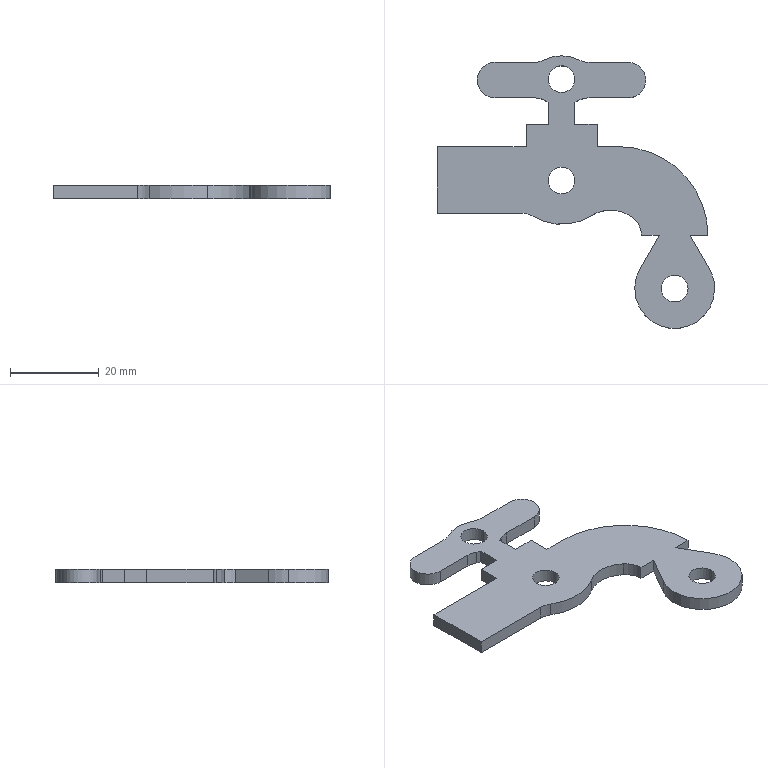Part | SolidWorks | features FlatPattern 1, ICE 1, SMBaseFlange 1, SheetMetal 1 | 1 solid | 44 faces | box 62.5 x 61.5 x 3 mm | volume 4665 mm3 | cylinder 24 | plane 20 | commonest cylinder face diameters 6 x6 10 x6 8 x3 17 x3 18 x3 16.181 x1
STEP:
#1=CARTESIAN_POINT('',(25.,30.211,-3.));
#2=VERTEX_POINT('',#1);
#3=CARTESIAN_POINT('',(31.,30.211,-3.));
#4=VERTEX_POINT('',#3);
#5=CARTESIAN_POINT('',(28.,30.211,-3.));
#6=DIRECTION('',(0.,0.,1.));
#7=DIRECTION('',(1.,0.,0.));
#8=AXIS2_PLACEMENT_3D('',#5,#6,#7);
#9=CIRCLE('',#8,3.);
#10=EDGE_CURVE('',#2,#4,#9,.T.);
#11=ORIENTED_EDGE('',*,*,#10,.F.);
#12=CARTESIAN_POINT('',(25.,30.211,0.));
#13=VERTEX_POINT('',#12);
#14=CARTESIAN_POINT('',(25.,30.211,-10.));
#15=DIRECTION('',(0.,0.,1.));
#16=VECTOR('',#15,1000.);
#17=LINE('',#14,#16);
#18=EDGE_CURVE('',#2,#13,#17,.T.);
#19=ORIENTED_EDGE('',*,*,#18,.T.);
#20=CARTESIAN_POINT('',(31.,30.211,0.));
#21=VERTEX_POINT('',#20);
#22=CARTESIAN_POINT('',(28.,30.211,0.));
#23=DIRECTION('',(0.,0.,1.));
#24=DIRECTION('',(1.,0.,0.));
#25=AXIS2_PLACEMENT_3D('',#22,#23,#24);
#26=CIRCLE('',#25,3.);
#27=EDGE_CURVE('',#13,#21,#26,.T.);
#28=ORIENTED_EDGE('',*,*,#27,.T.);
#29=CARTESIAN_POINT('',(31.,30.211,-10.));
#30=DIRECTION('',(0.,0.,1.));
#31=VECTOR('',#30,1000.);
#32=LINE('',#29,#31);
#33=EDGE_CURVE('',#4,#21,#32,.T.);
#34=ORIENTED_EDGE('',*,*,#33,.F.);
#35=EDGE_LOOP('',(#11,#19,#28,#34));
#36=FACE_OUTER_BOUND('',#35,.T.);
#37=CARTESIAN_POINT('',(28.,30.211,-10.));
#38=DIRECTION('',(0.,0.,1.));
#39=DIRECTION('',(1.,0.,0.));
#40=AXIS2_PLACEMENT_3D('',#37,#38,#39);
#41=CYLINDRICAL_SURFACE('',#40,3.);
#42=ADVANCED_FACE('',(#36),#41,.F.);
#43=CARTESIAN_POINT('',(25.,7.369,-3.));
#44=VERTEX_POINT('',#43);
#45=CARTESIAN_POINT('',(31.,7.369,-3.));
#46=VERTEX_POINT('',#45);
#47=CARTESIAN_POINT('',(28.,7.369,-3.));
#48=DIRECTION('',(0.,0.,1.));
#49=DIRECTION('',(1.,0.,0.));
#50=AXIS2_PLACEMENT_3D('',#47,#48,#49);
#51=CIRCLE('',#50,3.);
#52=EDGE_CURVE('',#44,#46,#51,.T.);
#53=ORIENTED_EDGE('',*,*,#52,.F.);
#54=CARTESIAN_POINT('',(25.,7.369,0.));
#55=VERTEX_POINT('',#54);
#56=CARTESIAN_POINT('',(25.,7.369,-10.));
#57=DIRECTION('',(0.,0.,1.));
#58=VECTOR('',#57,1000.);
#59=LINE('',#56,#58);
#60=EDGE_CURVE('',#44,#55,#59,.T.);
#61=ORIENTED_EDGE('',*,*,#60,.T.);
#62=CARTESIAN_POINT('',(31.,7.369,0.));
#63=VERTEX_POINT('',#62);
#64=CARTESIAN_POINT('',(28.,7.369,0.));
#65=DIRECTION('',(0.,0.,1.));
#66=DIRECTION('',(1.,0.,0.));
#67=AXIS2_PLACEMENT_3D('',#64,#65,#66);
#68=CIRCLE('',#67,3.);
#69=EDGE_CURVE('',#55,#63,#68,.T.);
#70=ORIENTED_EDGE('',*,*,#69,.T.);
#71=CARTESIAN_POINT('',(31.,7.369,-10.));
#72=DIRECTION('',(0.,0.,1.));
#73=VECTOR('',#72,1000.);
#74=LINE('',#71,#73);
#75=EDGE_CURVE('',#46,#63,#74,.T.);
#76=ORIENTED_EDGE('',*,*,#75,.F.);
#77=EDGE_LOOP('',(#53,#61,#70,#76));
#78=FACE_OUTER_BOUND('',#77,.T.);
#79=CARTESIAN_POINT('',(28.,7.369,-10.));
#80=DIRECTION('',(0.,0.,1.));
#81=DIRECTION('',(1.,0.,0.));
#82=AXIS2_PLACEMENT_3D('',#79,#80,#81);
#83=CYLINDRICAL_SURFACE('',#82,3.);
#84=ADVANCED_FACE('',(#78),#83,.F.);
#85=CARTESIAN_POINT('',(50.5,-17.,-3.));
#86=VERTEX_POINT('',#85);
#87=CARTESIAN_POINT('',(56.5,-17.,-3.));
#88=VERTEX_POINT('',#87);
#89=CARTESIAN_POINT('',(53.5,-17.,-3.));
#90=DIRECTION('',(0.,0.,1.));
#91=DIRECTION('',(1.,0.,0.));
#92=AXIS2_PLACEMENT_3D('',#89,#90,#91);
#93=CIRCLE('',#92,3.);
#94=EDGE_CURVE('',#86,#88,#93,.T.);
#95=ORIENTED_EDGE('',*,*,#94,.F.);
#96=CARTESIAN_POINT('',(50.5,-17.,0.));
#97=VERTEX_POINT('',#96);
#98=CARTESIAN_POINT('',(50.5,-17.,-10.));
#99=DIRECTION('',(0.,0.,1.));
#100=VECTOR('',#99,1000.);
#101=LINE('',#98,#100);
#102=EDGE_CURVE('',#86,#97,#101,.T.);
#103=ORIENTED_EDGE('',*,*,#102,.T.);
#104=CARTESIAN_POINT('',(56.5,-17.,0.));
#105=VERTEX_POINT('',#104);
#106=CARTESIAN_POINT('',(53.5,-17.,0.));
#107=DIRECTION('',(0.,0.,1.));
#108=DIRECTION('',(1.,0.,0.));
#109=AXIS2_PLACEMENT_3D('',#106,#107,#108);
#110=CIRCLE('',#109,3.);
#111=EDGE_CURVE('',#97,#105,#110,.T.);
#112=ORIENTED_EDGE('',*,*,#111,.T.);
#113=CARTESIAN_POINT('',(56.5,-17.,-10.));
#114=DIRECTION('',(0.,0.,1.));
#115=VECTOR('',#114,1000.);
#116=LINE('',#113,#115);
#117=EDGE_CURVE('',#88,#105,#116,.T.);
#118=ORIENTED_EDGE('',*,*,#117,.F.);
#119=EDGE_LOOP('',(#95,#103,#112,#118));
#120=FACE_OUTER_BOUND('',#119,.T.);
#121=CARTESIAN_POINT('',(53.5,-17.,-10.));
#122=DIRECTION('',(0.,0.,1.));
#123=DIRECTION('',(1.,0.,0.));
#124=AXIS2_PLACEMENT_3D('',#121,#122,#123);
#125=CYLINDRICAL_SURFACE('',#124,3.);
#126=ADVANCED_FACE('',(#120),#125,.F.);
#127=CARTESIAN_POINT('',(45.706,-12.5,-3.));
#128=VERTEX_POINT('',#127);
#129=CARTESIAN_POINT('',(44.5,-17.,-3.));
#130=VERTEX_POINT('',#129);
#131=CARTESIAN_POINT('',(53.5,-17.,-3.));
#132=DIRECTION('',(0.,0.,1.));
#133=DIRECTION('',(1.,0.,0.));
#134=AXIS2_PLACEMENT_3D('',#131,#132,#133);
#135=CIRCLE('',#134,9.);
#136=EDGE_CURVE('',#128,#130,#135,.T.);
#137=ORIENTED_EDGE('',*,*,#136,.T.);
#138=CARTESIAN_POINT('',(44.5,-17.,0.));
#139=VERTEX_POINT('',#138);
#140=CARTESIAN_POINT('',(44.5,-17.,-3.));
#141=DIRECTION('',(0.,0.,1.));
#142=VECTOR('',#141,1000.);
#143=LINE('',#140,#142);
#144=EDGE_CURVE('',#130,#139,#143,.T.);
#145=ORIENTED_EDGE('',*,*,#144,.T.);
#146=CARTESIAN_POINT('',(45.706,-12.5,0.));
#147=VERTEX_POINT('',#146);
#148=CARTESIAN_POINT('',(53.5,-17.,0.));
#149=DIRECTION('',(0.,0.,1.));
#150=DIRECTION('',(1.,0.,0.));
#151=AXIS2_PLACEMENT_3D('',#148,#149,#150);
#152=CIRCLE('',#151,9.);
#153=EDGE_CURVE('',#147,#139,#152,.T.);
#154=ORIENTED_EDGE('',*,*,#153,.F.);
#155=CARTESIAN_POINT('',(45.706,-12.5,-3.));
#156=DIRECTION('',(0.,0.,1.));
#157=VECTOR('',#156,1000.);
#158=LINE('',#155,#157);
#159=EDGE_CURVE('',#128,#147,#158,.T.);
#160=ORIENTED_EDGE('',*,*,#159,.F.);
#161=EDGE_LOOP('',(#137,#145,#154,#160));
#162=FACE_OUTER_BOUND('',#161,.T.);
#163=CARTESIAN_POINT('',(53.5,-17.,-3.));
#164=DIRECTION('',(0.,0.,1.));
#165=DIRECTION('',(1.,0.,0.));
#166=AXIS2_PLACEMENT_3D('',#163,#164,#165);
#167=CYLINDRICAL_SURFACE('',#166,9.);
#168=ADVANCED_FACE('',(#162),#167,.T.);
#169=ORIENTED_EDGE('',*,*,#144,.F.);
#170=CARTESIAN_POINT('',(62.5,-17.,-3.));
#171=VERTEX_POINT('',#170);
#172=CARTESIAN_POINT('',(53.5,-17.,-3.));
#173=DIRECTION('',(0.,0.,1.));
#174=DIRECTION('',(1.,0.,0.));
#175=AXIS2_PLACEMENT_3D('',#172,#173,#174);
#176=CIRCLE('',#175,9.);
#177=EDGE_CURVE('',#130,#171,#176,.T.);
#178=ORIENTED_EDGE('',*,*,#177,.T.);
#179=CARTESIAN_POINT('',(62.5,-17.,0.));
#180=VERTEX_POINT('',#179);
#181=CARTESIAN_POINT('',(62.5,-17.,-3.));
#182=DIRECTION('',(0.,0.,1.));
#183=VECTOR('',#182,1000.);
#184=LINE('',#181,#183);
#185=EDGE_CURVE('',#171,#180,#184,.T.);
#186=ORIENTED_EDGE('',*,*,#185,.T.);
#187=CARTESIAN_POINT('',(53.5,-17.,0.));
#188=DIRECTION('',(0.,0.,1.));
#189=DIRECTION('',(1.,0.,0.));
#190=AXIS2_PLACEMENT_3D('',#187,#188,#189);
#191=CIRCLE('',#190,9.);
#192=EDGE_CURVE('',#139,#180,#191,.T.);
#193=ORIENTED_EDGE('',*,*,#192,.F.);
#194=EDGE_LOOP('',(#169,#178,#186,#193));
#195=FACE_OUTER_BOUND('',#194,.T.);
#196=CARTESIAN_POINT('',(53.5,-17.,-3.));
#197=DIRECTION('',(0.,0.,1.));
#198=DIRECTION('',(1.,0.,0.));
#199=AXIS2_PLACEMENT_3D('',#196,#197,#198);
#200=CYLINDRICAL_SURFACE('',#199,9.);
#201=ADVANCED_FACE('',(#195),#200,.T.);
#202=CARTESIAN_POINT('',(43.,26.,-3.));
#203=VERTEX_POINT('',#202);
#204=CARTESIAN_POINT('',(47.,30.,-3.));
#205=VERTEX_POINT('',#204);
#206=CARTESIAN_POINT('',(43.,30.,-3.));
#207=DIRECTION('',(0.,0.,1.));
#208=DIRECTION('',(1.,0.,0.));
#209=AXIS2_PLACEMENT_3D('',#206,#207,#208);
#210=CIRCLE('',#209,4.);
#211=EDGE_CURVE('',#203,#205,#210,.T.);
#212=ORIENTED_EDGE('',*,*,#211,.T.);
#213=CARTESIAN_POINT('',(47.,30.,0.));
#214=VERTEX_POINT('',#213);
#215=CARTESIAN_POINT('',(47.,30.,-3.));
#216=DIRECTION('',(0.,0.,1.));
#217=VECTOR('',#216,1000.);
#218=LINE('',#215,#217);
#219=EDGE_CURVE('',#205,#214,#218,.T.);
#220=ORIENTED_EDGE('',*,*,#219,.T.);
#221=CARTESIAN_POINT('',(43.,26.,0.));
#222=VERTEX_POINT('',#221);
#223=CARTESIAN_POINT('',(43.,30.,0.));
#224=DIRECTION('',(0.,0.,1.));
#225=DIRECTION('',(1.,0.,0.));
#226=AXIS2_PLACEMENT_3D('',#223,#224,#225);
#227=CIRCLE('',#226,4.);
#228=EDGE_CURVE('',#222,#214,#227,.T.);
#229=ORIENTED_EDGE('',*,*,#228,.F.);
#230=CARTESIAN_POINT('',(43.,26.,-3.));
#231=DIRECTION('',(0.,0.,1.));
#232=VECTOR('',#231,1000.);
#233=LINE('',#230,#232);
#234=EDGE_CURVE('',#203,#222,#233,.T.);
#235=ORIENTED_EDGE('',*,*,#234,.F.);
#236=EDGE_LOOP('',(#212,#220,#229,#235));
#237=FACE_OUTER_BOUND('',#236,.T.);
#238=CARTESIAN_POINT('',(43.,30.,-3.));
#239=DIRECTION('',(0.,0.,1.));
#240=DIRECTION('',(1.,0.,0.));
#241=AXIS2_PLACEMENT_3D('',#238,#239,#240);
#242=CYLINDRICAL_SURFACE('',#241,4.);
#243=ADVANCED_FACE('',(#237),#242,.T.);
#244=CARTESIAN_POINT('',(0.,0.,0.));
#245=VERTEX_POINT('',#244);
#246=CARTESIAN_POINT('',(18.986,0.,0.));
#247=VERTEX_POINT('',#246);
#248=CARTESIAN_POINT('',(0.,0.,0.));
#249=DIRECTION('',(1.,0.,0.));
#250=VECTOR('',#249,1000.);
#251=LINE('',#248,#250);
#252=EDGE_CURVE('',#245,#247,#251,.T.);
#253=ORIENTED_EDGE('',*,*,#252,.F.);
#254=CARTESIAN_POINT('',(0.,0.,-3.));
#255=VERTEX_POINT('',#254);
#256=CARTESIAN_POINT('',(0.,0.,-3.));
#257=DIRECTION('',(0.,0.,1.));
#258=VECTOR('',#257,1000.);
#259=LINE('',#256,#258);
#260=EDGE_CURVE('',#255,#245,#259,.T.);
#261=ORIENTED_EDGE('',*,*,#260,.F.);
#262=CARTESIAN_POINT('',(18.986,0.,-3.));
#263=VERTEX_POINT('',#262);
#264=CARTESIAN_POINT('',(0.,0.,-3.));
#265=DIRECTION('',(1.,0.,0.));
#266=VECTOR('',#265,1000.);
#267=LINE('',#264,#266);
#268=EDGE_CURVE('',#255,#263,#267,.T.);
#269=ORIENTED_EDGE('',*,*,#268,.T.);
#270=CARTESIAN_POINT('',(18.986,0.,-3.));
#271=DIRECTION('',(0.,0.,1.));
#272=VECTOR('',#271,1000.);
#273=LINE('',#270,#272);
#274=EDGE_CURVE('',#263,#247,#273,.T.);
#275=ORIENTED_EDGE('',*,*,#274,.T.);
#276=EDGE_LOOP('',(#253,#261,#269,#275));
#277=FACE_OUTER_BOUND('',#276,.T.);
#278=CARTESIAN_POINT('',(0.,0.,-3.));
#279=DIRECTION('',(0.,-1.,0.));
#280=DIRECTION('',(0.,0.,-1.));
#281=AXIS2_PLACEMENT_3D('',#278,#279,#280);
#282=PLANE('',#281);
#283=ADVANCED_FACE('',(#277),#282,.T.);
#284=CARTESIAN_POINT('',(0.,15.,0.));
#285=VERTEX_POINT('',#284);
#286=CARTESIAN_POINT('',(0.,0.,0.));
#287=DIRECTION('',(0.,-1.,0.));
#288=VECTOR('',#287,1000.);
#289=LINE('',#286,#288);
#290=EDGE_CURVE('',#285,#245,#289,.T.);
#291=ORIENTED_EDGE('',*,*,#290,.F.);
#292=CARTESIAN_POINT('',(0.,15.,-3.));
#293=VERTEX_POINT('',#292);
#294=CARTESIAN_POINT('',(0.,15.,-3.));
#295=DIRECTION('',(0.,0.,1.));
#296=VECTOR('',#295,1000.);
#297=LINE('',#294,#296);
#298=EDGE_CURVE('',#293,#285,#297,.T.);
#299=ORIENTED_EDGE('',*,*,#298,.F.);
#300=CARTESIAN_POINT('',(0.,0.,-3.));
#301=DIRECTION('',(0.,-1.,0.));
#302=VECTOR('',#301,1000.);
#303=LINE('',#300,#302);
#304=EDGE_CURVE('',#293,#255,#303,.T.);
#305=ORIENTED_EDGE('',*,*,#304,.T.);
#306=ORIENTED_EDGE('',*,*,#260,.T.);
#307=EDGE_LOOP('',(#291,#299,#305,#306));
#308=FACE_OUTER_BOUND('',#307,.T.);
#309=CARTESIAN_POINT('',(0.,0.,-3.));
#310=DIRECTION('',(-1.,0.,0.));
#311=DIRECTION('',(0.,0.,1.));
#312=AXIS2_PLACEMENT_3D('',#309,#310,#311);
#313=PLANE('',#312);
#314=ADVANCED_FACE('',(#308),#313,.T.);
#315=CARTESIAN_POINT('',(20.,15.,0.));
#316=VERTEX_POINT('',#315);
#317=CARTESIAN_POINT('',(0.,15.,0.));
#318=DIRECTION('',(-1.,0.,0.));
#319=VECTOR('',#318,1000.);
#320=LINE('',#317,#319);
#321=EDGE_CURVE('',#316,#285,#320,.T.);
#322=ORIENTED_EDGE('',*,*,#321,.F.);
#323=CARTESIAN_POINT('',(20.,15.,-3.));
#324=VERTEX_POINT('',#323);
#325=CARTESIAN_POINT('',(20.,15.,-3.));
#326=DIRECTION('',(0.,0.,1.));
#327=VECTOR('',#326,1000.);
#328=LINE('',#325,#327);
#329=EDGE_CURVE('',#324,#316,#328,.T.);
#330=ORIENTED_EDGE('',*,*,#329,.F.);
#331=CARTESIAN_POINT('',(0.,15.,-3.));
#332=DIRECTION('',(-1.,0.,0.));
#333=VECTOR('',#332,1000.);
#334=LINE('',#331,#333);
#335=EDGE_CURVE('',#324,#293,#334,.T.);
#336=ORIENTED_EDGE('',*,*,#335,.T.);
#337=ORIENTED_EDGE('',*,*,#298,.T.);
#338=EDGE_LOOP('',(#322,#330,#336,#337));
#339=FACE_OUTER_BOUND('',#338,.T.);
#340=CARTESIAN_POINT('',(0.,15.,-3.));
#341=DIRECTION('',(0.,1.,0.));
#342=DIRECTION('',(0.,0.,1.));
#343=AXIS2_PLACEMENT_3D('',#340,#341,#342);
#344=PLANE('',#343);
#345=ADVANCED_FACE('',(#339),#344,.T.);
#346=CARTESIAN_POINT('',(20.,20.,0.));
#347=VERTEX_POINT('',#346);
#348=CARTESIAN_POINT('',(20.,15.,0.));
#349=DIRECTION('',(0.,-1.,0.));
#350=VECTOR('',#349,1000.);
#351=LINE('',#348,#350);
#352=EDGE_CURVE('',#347,#316,#351,.T.);
#353=ORIENTED_EDGE('',*,*,#352,.F.);
#354=CARTESIAN_POINT('',(20.,20.,-3.));
#355=VERTEX_POINT('',#354);
#356=CARTESIAN_POINT('',(20.,20.,-3.));
#357=DIRECTION('',(0.,0.,1.));
#358=VECTOR('',#357,1000.);
#359=LINE('',#356,#358);
#360=EDGE_CURVE('',#355,#347,#359,.T.);
#361=ORIENTED_EDGE('',*,*,#360,.F.);
#362=CARTESIAN_POINT('',(20.,15.,-3.));
#363=DIRECTION('',(0.,-1.,0.));
#364=VECTOR('',#363,1000.);
#365=LINE('',#362,#364);
#366=EDGE_CURVE('',#355,#324,#365,.T.);
#367=ORIENTED_EDGE('',*,*,#366,.T.);
#368=ORIENTED_EDGE('',*,*,#329,.T.);
#369=EDGE_LOOP('',(#353,#361,#367,#368));
#370=FACE_OUTER_BOUND('',#369,.T.);
#371=CARTESIAN_POINT('',(20.,15.,-3.));
#372=DIRECTION('',(-1.,0.,0.));
#373=DIRECTION('',(0.,0.,1.));
#374=AXIS2_PLACEMENT_3D('',#371,#372,#373);
#375=PLANE('',#374);
#376=ADVANCED_FACE('',(#370),#375,.T.);
#377=CARTESIAN_POINT('',(25.,20.,0.));
#378=VERTEX_POINT('',#377);
#379=CARTESIAN_POINT('',(20.,20.,0.));
#380=DIRECTION('',(-1.,0.,0.));
#381=VECTOR('',#380,1000.);
#382=LINE('',#379,#381);
#383=EDGE_CURVE('',#378,#347,#382,.T.);
#384=ORIENTED_EDGE('',*,*,#383,.F.);
#385=CARTESIAN_POINT('',(25.,20.,-3.));
#386=VERTEX_POINT('',#385);
#387=CARTESIAN_POINT('',(25.,20.,-3.));
#388=DIRECTION('',(0.,0.,1.));
#389=VECTOR('',#388,1000.);
#390=LINE('',#387,#389);
#391=EDGE_CURVE('',#386,#378,#390,.T.);
#392=ORIENTED_EDGE('',*,*,#391,.F.);
#393=CARTESIAN_POINT('',(20.,20.,-3.));
#394=DIRECTION('',(-1.,0.,0.));
#395=VECTOR('',#394,1000.);
#396=LINE('',#393,#395);
#397=EDGE_CURVE('',#386,#355,#396,.T.);
#398=ORIENTED_EDGE('',*,*,#397,.T.);
#399=ORIENTED_EDGE('',*,*,#360,.T.);
#400=EDGE_LOOP('',(#384,#392,#398,#399));
#401=FACE_OUTER_BOUND('',#400,.T.);
#402=CARTESIAN_POINT('',(20.,20.,-3.));
#403=DIRECTION('',(0.,1.,0.));
#404=DIRECTION('',(0.,0.,1.));
#405=AXIS2_PLACEMENT_3D('',#402,#403,#404);
#406=PLANE('',#405);
#407=ADVANCED_FACE('',(#401),#406,.T.);
#408=CARTESIAN_POINT('',(25.,25.047,0.));
#409=VERTEX_POINT('',#408);
#410=CARTESIAN_POINT('',(25.,20.,0.));
#411=DIRECTION('',(0.,-1.,0.));
#412=VECTOR('',#411,1000.);
#413=LINE('',#410,#412);
#414=EDGE_CURVE('',#409,#378,#413,.T.);
#415=ORIENTED_EDGE('',*,*,#414,.F.);
#416=CARTESIAN_POINT('',(25.,25.047,-3.));
#417=VERTEX_POINT('',#416);
#418=CARTESIAN_POINT('',(25.,25.047,-3.));
#419=DIRECTION('',(0.,0.,1.));
#420=VECTOR('',#419,1000.);
#421=LINE('',#418,#420);
#422=EDGE_CURVE('',#417,#409,#421,.T.);
#423=ORIENTED_EDGE('',*,*,#422,.F.);
#424=CARTESIAN_POINT('',(25.,20.,-3.));
#425=DIRECTION('',(0.,-1.,0.));
#426=VECTOR('',#425,1000.);
#427=LINE('',#424,#426);
#428=EDGE_CURVE('',#417,#386,#427,.T.);
#429=ORIENTED_EDGE('',*,*,#428,.T.);
#430=ORIENTED_EDGE('',*,*,#391,.T.);
#431=EDGE_LOOP('',(#415,#423,#429,#430));
#432=FACE_OUTER_BOUND('',#431,.T.);
#433=CARTESIAN_POINT('',(25.,20.,-3.));
#434=DIRECTION('',(-1.,0.,0.));
#435=DIRECTION('',(0.,0.,1.));
#436=AXIS2_PLACEMENT_3D('',#433,#434,#435);
#437=PLANE('',#436);
#438=ADVANCED_FACE('',(#432),#437,.T.);
#439=CARTESIAN_POINT('',(24.106,25.444,0.));
#440=VERTEX_POINT('',#439);
#441=CARTESIAN_POINT('',(28.,33.,0.));
#442=DIRECTION('',(0.,0.,1.));
#443=DIRECTION('',(1.,0.,0.));
#444=AXIS2_PLACEMENT_3D('',#441,#442,#443);
#445=CIRCLE('',#444,8.5);
#446=EDGE_CURVE('',#440,#409,#445,.T.);
#447=ORIENTED_EDGE('',*,*,#446,.F.);
#448=CARTESIAN_POINT('',(24.106,25.444,-3.));
#449=VERTEX_POINT('',#448);
#450=CARTESIAN_POINT('',(24.106,25.444,-3.));
#451=DIRECTION('',(0.,0.,1.));
#452=VECTOR('',#451,1000.);
#453=LINE('',#450,#452);
#454=EDGE_CURVE('',#449,#440,#453,.T.);
#455=ORIENTED_EDGE('',*,*,#454,.F.);
#456=CARTESIAN_POINT('',(28.,33.,-3.));
#457=DIRECTION('',(0.,0.,1.));
#458=DIRECTION('',(1.,0.,0.));
#459=AXIS2_PLACEMENT_3D('',#456,#457,#458);
#460=CIRCLE('',#459,8.5);
#461=EDGE_CURVE('',#449,#417,#460,.T.);
#462=ORIENTED_EDGE('',*,*,#461,.T.);
#463=ORIENTED_EDGE('',*,*,#422,.T.);
#464=EDGE_LOOP('',(#447,#455,#462,#463));
#465=FACE_OUTER_BOUND('',#464,.T.);
#466=CARTESIAN_POINT('',(28.,33.,-3.));
#467=DIRECTION('',(0.,0.,1.));
#468=DIRECTION('',(1.,0.,0.));
#469=AXIS2_PLACEMENT_3D('',#466,#467,#468);
#470=CYLINDRICAL_SURFACE('',#469,8.5);
#471=ADVANCED_FACE('',(#465),#470,.T.);
#472=CARTESIAN_POINT('',(21.815,26.,0.));
#473=VERTEX_POINT('',#472);
#474=CARTESIAN_POINT('',(21.815,21.,0.));
#475=DIRECTION('',(0.,0.,-1.));
#476=DIRECTION('',(1.,0.,0.));
#477=AXIS2_PLACEMENT_3D('',#474,#475,#476);
#478=CIRCLE('',#477,5.);
#479=EDGE_CURVE('',#473,#440,#478,.T.);
#480=ORIENTED_EDGE('',*,*,#479,.F.);
#481=CARTESIAN_POINT('',(21.815,26.,-3.));
#482=VERTEX_POINT('',#481);
#483=CARTESIAN_POINT('',(21.815,26.,-3.));
#484=DIRECTION('',(0.,0.,1.));
#485=VECTOR('',#484,1000.);
#486=LINE('',#483,#485);
#487=EDGE_CURVE('',#482,#473,#486,.T.);
#488=ORIENTED_EDGE('',*,*,#487,.F.);
#489=CARTESIAN_POINT('',(21.815,21.,-3.));
#490=DIRECTION('',(0.,0.,-1.));
#491=DIRECTION('',(1.,0.,0.));
#492=AXIS2_PLACEMENT_3D('',#489,#490,#491);
#493=CIRCLE('',#492,5.);
#494=EDGE_CURVE('',#482,#449,#493,.T.);
#495=ORIENTED_EDGE('',*,*,#494,.T.);
#496=ORIENTED_EDGE('',*,*,#454,.T.);
#497=EDGE_LOOP('',(#480,#488,#495,#496));
#498=FACE_OUTER_BOUND('',#497,.T.);
#499=CARTESIAN_POINT('',(21.815,21.,-3.));
#500=DIRECTION('',(0.,0.,1.));
#501=DIRECTION('',(1.,0.,0.));
#502=AXIS2_PLACEMENT_3D('',#499,#500,#501);
#503=CYLINDRICAL_SURFACE('',#502,5.);
#504=ADVANCED_FACE('',(#498),#503,.F.);
#505=CARTESIAN_POINT('',(13.,26.,0.));
#506=VERTEX_POINT('',#505);
#507=CARTESIAN_POINT('',(13.,26.,0.));
#508=DIRECTION('',(1.,0.,0.));
#509=VECTOR('',#508,1000.);
#510=LINE('',#507,#509);
#511=EDGE_CURVE('',#506,#473,#510,.T.);
#512=ORIENTED_EDGE('',*,*,#511,.F.);
#513=CARTESIAN_POINT('',(13.,26.,-3.));
#514=VERTEX_POINT('',#513);
#515=CARTESIAN_POINT('',(13.,26.,-3.));
#516=DIRECTION('',(0.,0.,1.));
#517=VECTOR('',#516,1000.);
#518=LINE('',#515,#517);
#519=EDGE_CURVE('',#514,#506,#518,.T.);
#520=ORIENTED_EDGE('',*,*,#519,.F.);
#521=CARTESIAN_POINT('',(13.,26.,-3.));
#522=DIRECTION('',(1.,0.,0.));
#523=VECTOR('',#522,1000.);
#524=LINE('',#521,#523);
#525=EDGE_CURVE('',#514,#482,#524,.T.);
#526=ORIENTED_EDGE('',*,*,#525,.T.);
#527=ORIENTED_EDGE('',*,*,#487,.T.);
#528=EDGE_LOOP('',(#512,#520,#526,#527));
#529=FACE_OUTER_BOUND('',#528,.T.);
#530=CARTESIAN_POINT('',(13.,26.,-3.));
#531=DIRECTION('',(0.,-1.,0.));
#532=DIRECTION('',(0.,0.,-1.));
#533=AXIS2_PLACEMENT_3D('',#530,#531,#532);
#534=PLANE('',#533);
#535=ADVANCED_FACE('',(#529),#534,.T.);
#536=CARTESIAN_POINT('',(13.,34.,0.));
#537=VERTEX_POINT('',#536);
#538=CARTESIAN_POINT('',(13.,30.,0.));
#539=DIRECTION('',(0.,0.,1.));
#540=DIRECTION('',(1.,0.,0.));
#541=AXIS2_PLACEMENT_3D('',#538,#539,#540);
#542=CIRCLE('',#541,4.);
#543=EDGE_CURVE('',#537,#506,#542,.T.);
#544=ORIENTED_EDGE('',*,*,#543,.F.);
#545=CARTESIAN_POINT('',(13.,34.,-3.));
#546=VERTEX_POINT('',#545);
#547=CARTESIAN_POINT('',(13.,34.,-3.));
#548=DIRECTION('',(0.,0.,1.));
#549=VECTOR('',#548,1000.);
#550=LINE('',#547,#549);
#551=EDGE_CURVE('',#546,#537,#550,.T.);
#552=ORIENTED_EDGE('',*,*,#551,.F.);
#553=CARTESIAN_POINT('',(13.,30.,-3.));
#554=DIRECTION('',(0.,0.,1.));
#555=DIRECTION('',(1.,0.,0.));
#556=AXIS2_PLACEMENT_3D('',#553,#554,#555);
#557=CIRCLE('',#556,4.);
#558=EDGE_CURVE('',#546,#514,#557,.T.);
#559=ORIENTED_EDGE('',*,*,#558,.T.);
#560=ORIENTED_EDGE('',*,*,#519,.T.);
#561=EDGE_LOOP('',(#544,#552,#559,#560));
#562=FACE_OUTER_BOUND('',#561,.T.);
#563=CARTESIAN_POINT('',(13.,30.,-3.));
#564=DIRECTION('',(0.,0.,1.));
#565=DIRECTION('',(1.,0.,0.));
#566=AXIS2_PLACEMENT_3D('',#563,#564,#565);
#567=CYLINDRICAL_SURFACE('',#566,4.);
#568=ADVANCED_FACE('',(#562),#567,.T.);
#569=CARTESIAN_POINT('',(21.815,34.,0.));
#570=VERTEX_POINT('',#569);
#571=CARTESIAN_POINT('',(13.,34.,0.));
#572=DIRECTION('',(-1.,0.,0.));
#573=VECTOR('',#572,1000.);
#574=LINE('',#571,#573);
#575=EDGE_CURVE('',#570,#537,#574,.T.);
#576=ORIENTED_EDGE('',*,*,#575,.F.);
#577=CARTESIAN_POINT('',(21.815,34.,-3.));
#578=VERTEX_POINT('',#577);
#579=CARTESIAN_POINT('',(21.815,34.,-3.));
#580=DIRECTION('',(0.,0.,1.));
#581=VECTOR('',#580,1000.);
#582=LINE('',#579,#581);
#583=EDGE_CURVE('',#578,#570,#582,.T.);
#584=ORIENTED_EDGE('',*,*,#583,.F.);
#585=CARTESIAN_POINT('',(13.,34.,-3.));
#586=DIRECTION('',(-1.,0.,0.));
#587=VECTOR('',#586,1000.);
#588=LINE('',#585,#587);
#589=EDGE_CURVE('',#578,#546,#588,.T.);
#590=ORIENTED_EDGE('',*,*,#589,.T.);
#591=ORIENTED_EDGE('',*,*,#551,.T.);
#592=EDGE_LOOP('',(#576,#584,#590,#591));
#593=FACE_OUTER_BOUND('',#592,.T.);
#594=CARTESIAN_POINT('',(13.,34.,-3.));
#595=DIRECTION('',(0.,1.,0.));
#596=DIRECTION('',(-1.,0.,0.));
#597=AXIS2_PLACEMENT_3D('',#594,#595,#596);
#598=PLANE('',#597);
#599=ADVANCED_FACE('',(#593),#598,.T.);
#600=CARTESIAN_POINT('',(24.106,34.556,0.));
#601=VERTEX_POINT('',#600);
#602=CARTESIAN_POINT('',(21.815,39.,0.));
#603=DIRECTION('',(0.,0.,-1.));
#604=DIRECTION('',(-1.,0.,0.));
#605=AXIS2_PLACEMENT_3D('',#602,#603,#604);
#606=CIRCLE('',#605,5.);
#607=EDGE_CURVE('',#601,#570,#606,.T.);
#608=ORIENTED_EDGE('',*,*,#607,.F.);
#609=CARTESIAN_POINT('',(24.106,34.556,-3.));
#610=VERTEX_POINT('',#609);
#611=CARTESIAN_POINT('',(24.106,34.556,-3.));
#612=DIRECTION('',(0.,0.,1.));
#613=VECTOR('',#612,1000.);
#614=LINE('',#611,#613);
#615=EDGE_CURVE('',#610,#601,#614,.T.);
#616=ORIENTED_EDGE('',*,*,#615,.F.);
#617=CARTESIAN_POINT('',(21.815,39.,-3.));
#618=DIRECTION('',(0.,0.,-1.));
#619=DIRECTION('',(-1.,0.,0.));
#620=AXIS2_PLACEMENT_3D('',#617,#618,#619);
#621=CIRCLE('',#620,5.);
#622=EDGE_CURVE('',#610,#578,#621,.T.);
#623=ORIENTED_EDGE('',*,*,#622,.T.);
#624=ORIENTED_EDGE('',*,*,#583,.T.);
#625=EDGE_LOOP('',(#608,#616,#623,#624));
#626=FACE_OUTER_BOUND('',#625,.T.);
#627=CARTESIAN_POINT('',(21.815,39.,-3.));
#628=DIRECTION('',(0.,0.,1.));
#629=DIRECTION('',(1.,0.,0.));
#630=AXIS2_PLACEMENT_3D('',#627,#628,#629);
#631=CYLINDRICAL_SURFACE('',#630,5.);
#632=ADVANCED_FACE('',(#626),#631,.F.);
#633=CARTESIAN_POINT('',(31.894,34.556,0.));
#634=VERTEX_POINT('',#633);
#635=CARTESIAN_POINT('',(28.,27.,0.));
#636=DIRECTION('',(0.,0.,1.));
#637=DIRECTION('',(1.,0.,0.));
#638=AXIS2_PLACEMENT_3D('',#635,#636,#637);
#639=CIRCLE('',#638,8.5);
#640=EDGE_CURVE('',#634,#601,#639,.T.);
#641=ORIENTED_EDGE('',*,*,#640,.F.);
#642=CARTESIAN_POINT('',(31.894,34.556,-3.));
#643=VERTEX_POINT('',#642);
#644=CARTESIAN_POINT('',(31.894,34.556,-3.));
#645=DIRECTION('',(0.,0.,1.));
#646=VECTOR('',#645,1000.);
#647=LINE('',#644,#646);
#648=EDGE_CURVE('',#643,#634,#647,.T.);
#649=ORIENTED_EDGE('',*,*,#648,.F.);
#650=CARTESIAN_POINT('',(28.,27.,-3.));
#651=DIRECTION('',(0.,0.,1.));
#652=DIRECTION('',(1.,0.,0.));
#653=AXIS2_PLACEMENT_3D('',#650,#651,#652);
#654=CIRCLE('',#653,8.5);
#655=EDGE_CURVE('',#643,#610,#654,.T.);
#656=ORIENTED_EDGE('',*,*,#655,.T.);
#657=ORIENTED_EDGE('',*,*,#615,.T.);
#658=EDGE_LOOP('',(#641,#649,#656,#657));
#659=FACE_OUTER_BOUND('',#658,.T.);
#660=CARTESIAN_POINT('',(28.,27.,-3.));
#661=DIRECTION('',(0.,0.,1.));
#662=DIRECTION('',(1.,0.,0.));
#663=AXIS2_PLACEMENT_3D('',#660,#661,#662);
#664=CYLINDRICAL_SURFACE('',#663,8.5);
#665=ADVANCED_FACE('',(#659),#664,.T.);
#666=CARTESIAN_POINT('',(34.185,34.,0.));
#667=VERTEX_POINT('',#666);
#668=CARTESIAN_POINT('',(34.185,39.,0.));
#669=DIRECTION('',(0.,0.,-1.));
#670=DIRECTION('',(1.,0.,0.));
#671=AXIS2_PLACEMENT_3D('',#668,#669,#670);
#672=CIRCLE('',#671,5.);
#673=EDGE_CURVE('',#667,#634,#672,.T.);
#674=ORIENTED_EDGE('',*,*,#673,.F.);
#675=CARTESIAN_POINT('',(34.185,34.,-3.));
#676=VERTEX_POINT('',#675);
#677=CARTESIAN_POINT('',(34.185,34.,-3.));
#678=DIRECTION('',(0.,0.,1.));
#679=VECTOR('',#678,1000.);
#680=LINE('',#677,#679);
#681=EDGE_CURVE('',#676,#667,#680,.T.);
#682=ORIENTED_EDGE('',*,*,#681,.F.);
#683=CARTESIAN_POINT('',(34.185,39.,-3.));
#684=DIRECTION('',(0.,0.,-1.));
#685=DIRECTION('',(1.,0.,0.));
#686=AXIS2_PLACEMENT_3D('',#683,#684,#685);
#687=CIRCLE('',#686,5.);
#688=EDGE_CURVE('',#676,#643,#687,.T.);
#689=ORIENTED_EDGE('',*,*,#688,.T.);
#690=ORIENTED_EDGE('',*,*,#648,.T.);
#691=EDGE_LOOP('',(#674,#682,#689,#690));
#692=FACE_OUTER_BOUND('',#691,.T.);
#693=CARTESIAN_POINT('',(34.185,39.,-3.));
#694=DIRECTION('',(0.,0.,1.));
#695=DIRECTION('',(1.,0.,0.));
#696=AXIS2_PLACEMENT_3D('',#693,#694,#695);
#697=CYLINDRICAL_SURFACE('',#696,5.);
#698=ADVANCED_FACE('',(#692),#697,.F.);
#699=CARTESIAN_POINT('',(43.,34.,0.));
#700=VERTEX_POINT('',#699);
#701=CARTESIAN_POINT('',(34.185,34.,0.));
#702=DIRECTION('',(-1.,0.,0.));
#703=VECTOR('',#702,1000.);
#704=LINE('',#701,#703);
#705=EDGE_CURVE('',#700,#667,#704,.T.);
#706=ORIENTED_EDGE('',*,*,#705,.F.);
#707=CARTESIAN_POINT('',(43.,34.,-3.));
#708=VERTEX_POINT('',#707);
#709=CARTESIAN_POINT('',(43.,34.,-3.));
#710=DIRECTION('',(0.,0.,1.));
#711=VECTOR('',#710,1000.);
#712=LINE('',#709,#711);
#713=EDGE_CURVE('',#708,#700,#712,.T.);
#714=ORIENTED_EDGE('',*,*,#713,.F.);
#715=CARTESIAN_POINT('',(34.185,34.,-3.));
#716=DIRECTION('',(-1.,0.,0.));
#717=VECTOR('',#716,1000.);
#718=LINE('',#715,#717);
#719=EDGE_CURVE('',#708,#676,#718,.T.);
#720=ORIENTED_EDGE('',*,*,#719,.T.);
#721=ORIENTED_EDGE('',*,*,#681,.T.);
#722=EDGE_LOOP('',(#706,#714,#720,#721));
#723=FACE_OUTER_BOUND('',#722,.T.);
#724=CARTESIAN_POINT('',(34.185,34.,-3.));
#725=DIRECTION('',(0.,1.,0.));
#726=DIRECTION('',(0.,0.,1.));
#727=AXIS2_PLACEMENT_3D('',#724,#725,#726);
#728=PLANE('',#727);
#729=ADVANCED_FACE('',(#723),#728,.T.);
#730=ORIENTED_EDGE('',*,*,#219,.F.);
#731=CARTESIAN_POINT('',(43.,30.,-3.));
#732=DIRECTION('',(0.,0.,1.));
#733=DIRECTION('',(1.,0.,0.));
#734=AXIS2_PLACEMENT_3D('',#731,#732,#733);
#735=CIRCLE('',#734,4.);
#736=EDGE_CURVE('',#205,#708,#735,.T.);
#737=ORIENTED_EDGE('',*,*,#736,.T.);
#738=ORIENTED_EDGE('',*,*,#713,.T.);
#739=CARTESIAN_POINT('',(43.,30.,0.));
#740=DIRECTION('',(0.,0.,1.));
#741=DIRECTION('',(1.,0.,0.));
#742=AXIS2_PLACEMENT_3D('',#739,#740,#741);
#743=CIRCLE('',#742,4.);
#744=EDGE_CURVE('',#214,#700,#743,.T.);
#745=ORIENTED_EDGE('',*,*,#744,.F.);
#746=EDGE_LOOP('',(#730,#737,#738,#745));
#747=FACE_OUTER_BOUND('',#746,.T.);
#748=CARTESIAN_POINT('',(43.,30.,-3.));
#749=DIRECTION('',(0.,0.,1.));
#750=DIRECTION('',(1.,0.,0.));
#751=AXIS2_PLACEMENT_3D('',#748,#749,#750);
#752=CYLINDRICAL_SURFACE('',#751,4.);
#753=ADVANCED_FACE('',(#747),#752,.T.);
#754=CARTESIAN_POINT('',(34.185,26.,0.));
#755=VERTEX_POINT('',#754);
#756=CARTESIAN_POINT('',(34.185,26.,0.));
#757=DIRECTION('',(1.,0.,0.));
#758=VECTOR('',#757,1000.);
#759=LINE('',#756,#758);
#760=EDGE_CURVE('',#755,#222,#759,.T.);
#761=ORIENTED_EDGE('',*,*,#760,.F.);
#762=CARTESIAN_POINT('',(34.185,26.,-3.));
#763=VERTEX_POINT('',#762);
#764=CARTESIAN_POINT('',(34.185,26.,-3.));
#765=DIRECTION('',(0.,0.,1.));
#766=VECTOR('',#765,1000.);
#767=LINE('',#764,#766);
#768=EDGE_CURVE('',#763,#755,#767,.T.);
#769=ORIENTED_EDGE('',*,*,#768,.F.);
#770=CARTESIAN_POINT('',(34.185,26.,-3.));
#771=DIRECTION('',(1.,0.,0.));
#772=VECTOR('',#771,1000.);
#773=LINE('',#770,#772);
#774=EDGE_CURVE('',#763,#203,#773,.T.);
#775=ORIENTED_EDGE('',*,*,#774,.T.);
#776=ORIENTED_EDGE('',*,*,#234,.T.);
#777=EDGE_LOOP('',(#761,#769,#775,#776));
#778=FACE_OUTER_BOUND('',#777,.T.);
#779=CARTESIAN_POINT('',(34.185,26.,-3.));
#780=DIRECTION('',(0.,-1.,0.));
#781=DIRECTION('',(1.,0.,0.));
#782=AXIS2_PLACEMENT_3D('',#779,#780,#781);
#783=PLANE('',#782);
#784=ADVANCED_FACE('',(#778),#783,.T.);
#785=CARTESIAN_POINT('',(31.894,25.444,0.));
#786=VERTEX_POINT('',#785);
#787=CARTESIAN_POINT('',(34.185,21.,0.));
#788=DIRECTION('',(0.,0.,-1.));
#789=DIRECTION('',(-1.,0.,0.));
#790=AXIS2_PLACEMENT_3D('',#787,#788,#789);
#791=CIRCLE('',#790,5.);
#792=EDGE_CURVE('',#786,#755,#791,.T.);
#793=ORIENTED_EDGE('',*,*,#792,.F.);
#794=CARTESIAN_POINT('',(31.894,25.444,-3.));
#795=VERTEX_POINT('',#794);
#796=CARTESIAN_POINT('',(31.894,25.444,-3.));
#797=DIRECTION('',(0.,0.,1.));
#798=VECTOR('',#797,1000.);
#799=LINE('',#796,#798);
#800=EDGE_CURVE('',#795,#786,#799,.T.);
#801=ORIENTED_EDGE('',*,*,#800,.F.);
#802=CARTESIAN_POINT('',(34.185,21.,-3.));
#803=DIRECTION('',(0.,0.,-1.));
#804=DIRECTION('',(-1.,0.,0.));
#805=AXIS2_PLACEMENT_3D('',#802,#803,#804);
#806=CIRCLE('',#805,5.);
#807=EDGE_CURVE('',#795,#763,#806,.T.);
#808=ORIENTED_EDGE('',*,*,#807,.T.);
#809=ORIENTED_EDGE('',*,*,#768,.T.);
#810=EDGE_LOOP('',(#793,#801,#808,#809));
#811=FACE_OUTER_BOUND('',#810,.T.);
#812=CARTESIAN_POINT('',(34.185,21.,-3.));
#813=DIRECTION('',(0.,0.,1.));
#814=DIRECTION('',(1.,0.,0.));
#815=AXIS2_PLACEMENT_3D('',#812,#813,#814);
#816=CYLINDRICAL_SURFACE('',#815,5.);
#817=ADVANCED_FACE('',(#811),#816,.F.);
#818=CARTESIAN_POINT('',(31.,25.047,0.));
#819=VERTEX_POINT('',#818);
#820=CARTESIAN_POINT('',(28.,33.,0.));
#821=DIRECTION('',(0.,0.,1.));
#822=DIRECTION('',(1.,0.,0.));
#823=AXIS2_PLACEMENT_3D('',#820,#821,#822);
#824=CIRCLE('',#823,8.5);
#825=EDGE_CURVE('',#819,#786,#824,.T.);
#826=ORIENTED_EDGE('',*,*,#825,.F.);
#827=CARTESIAN_POINT('',(31.,25.047,-3.));
#828=VERTEX_POINT('',#827);
#829=CARTESIAN_POINT('',(31.,25.047,-3.));
#830=DIRECTION('',(0.,0.,1.));
#831=VECTOR('',#830,1000.);
#832=LINE('',#829,#831);
#833=EDGE_CURVE('',#828,#819,#832,.T.);
#834=ORIENTED_EDGE('',*,*,#833,.F.);
#835=CARTESIAN_POINT('',(28.,33.,-3.));
#836=DIRECTION('',(0.,0.,1.));
#837=DIRECTION('',(1.,0.,0.));
#838=AXIS2_PLACEMENT_3D('',#835,#836,#837);
#839=CIRCLE('',#838,8.5);
#840=EDGE_CURVE('',#828,#795,#839,.T.);
#841=ORIENTED_EDGE('',*,*,#840,.T.);
#842=ORIENTED_EDGE('',*,*,#800,.T.);
#843=EDGE_LOOP('',(#826,#834,#841,#842));
#844=FACE_OUTER_BOUND('',#843,.T.);
#845=CARTESIAN_POINT('',(28.,33.,-3.));
#846=DIRECTION('',(0.,0.,1.));
#847=DIRECTION('',(1.,0.,0.));
#848=AXIS2_PLACEMENT_3D('',#845,#846,#847);
#849=CYLINDRICAL_SURFACE('',#848,8.5);
#850=ADVANCED_FACE('',(#844),#849,.T.);
#851=CARTESIAN_POINT('',(31.,20.,0.));
#852=VERTEX_POINT('',#851);
#853=CARTESIAN_POINT('',(31.,25.047,0.));
#854=DIRECTION('',(0.,1.,0.));
#855=VECTOR('',#854,1000.);
#856=LINE('',#853,#855);
#857=EDGE_CURVE('',#852,#819,#856,.T.);
#858=ORIENTED_EDGE('',*,*,#857,.F.);
#859=CARTESIAN_POINT('',(31.,20.,-3.));
#860=VERTEX_POINT('',#859);
#861=CARTESIAN_POINT('',(31.,20.,-3.));
#862=DIRECTION('',(0.,0.,1.));
#863=VECTOR('',#862,1000.);
#864=LINE('',#861,#863);
#865=EDGE_CURVE('',#860,#852,#864,.T.);
#866=ORIENTED_EDGE('',*,*,#865,.F.);
#867=CARTESIAN_POINT('',(31.,25.047,-3.));
#868=DIRECTION('',(0.,1.,0.));
#869=VECTOR('',#868,1000.);
#870=LINE('',#867,#869);
#871=EDGE_CURVE('',#860,#828,#870,.T.);
#872=ORIENTED_EDGE('',*,*,#871,.T.);
#873=ORIENTED_EDGE('',*,*,#833,.T.);
#874=EDGE_LOOP('',(#858,#866,#872,#873));
#875=FACE_OUTER_BOUND('',#874,.T.);
#876=CARTESIAN_POINT('',(31.,25.047,-3.));
#877=DIRECTION('',(1.,0.,0.));
#878=DIRECTION('',(0.,1.,0.));
#879=AXIS2_PLACEMENT_3D('',#876,#877,#878);
#880=PLANE('',#879);
#881=ADVANCED_FACE('',(#875),#880,.T.);
#882=CARTESIAN_POINT('',(36.,20.,0.));
#883=VERTEX_POINT('',#882);
#884=CARTESIAN_POINT('',(31.,20.,0.));
#885=DIRECTION('',(-1.,0.,0.));
#886=VECTOR('',#885,1000.);
#887=LINE('',#884,#886);
#888=EDGE_CURVE('',#883,#852,#887,.T.);
#889=ORIENTED_EDGE('',*,*,#888,.F.);
#890=CARTESIAN_POINT('',(36.,20.,-3.));
#891=VERTEX_POINT('',#890);
#892=CARTESIAN_POINT('',(36.,20.,-3.));
#893=DIRECTION('',(0.,0.,1.));
#894=VECTOR('',#893,1000.);
#895=LINE('',#892,#894);
#896=EDGE_CURVE('',#891,#883,#895,.T.);
#897=ORIENTED_EDGE('',*,*,#896,.F.);
#898=CARTESIAN_POINT('',(31.,20.,-3.));
#899=DIRECTION('',(-1.,0.,0.));
#900=VECTOR('',#899,1000.);
#901=LINE('',#898,#900);
#902=EDGE_CURVE('',#891,#860,#901,.T.);
#903=ORIENTED_EDGE('',*,*,#902,.T.);
#904=ORIENTED_EDGE('',*,*,#865,.T.);
#905=EDGE_LOOP('',(#889,#897,#903,#904));
#906=FACE_OUTER_BOUND('',#905,.T.);
#907=CARTESIAN_POINT('',(31.,20.,-3.));
#908=DIRECTION('',(0.,1.,0.));
#909=DIRECTION('',(-1.,0.,0.));
#910=AXIS2_PLACEMENT_3D('',#907,#908,#909);
#911=PLANE('',#910);
#912=ADVANCED_FACE('',(#906),#911,.T.);
#913=CARTESIAN_POINT('',(36.,15.,0.));
#914=VERTEX_POINT('',#913);
#915=CARTESIAN_POINT('',(36.,20.,0.));
#916=DIRECTION('',(0.,1.,0.));
#917=VECTOR('',#916,1000.);
#918=LINE('',#915,#917);
#919=EDGE_CURVE('',#914,#883,#918,.T.);
#920=ORIENTED_EDGE('',*,*,#919,.F.);
#921=CARTESIAN_POINT('',(36.,15.,-3.));
#922=VERTEX_POINT('',#921);
#923=CARTESIAN_POINT('',(36.,15.,-3.));
#924=DIRECTION('',(0.,0.,1.));
#925=VECTOR('',#924,1000.);
#926=LINE('',#923,#925);
#927=EDGE_CURVE('',#922,#914,#926,.T.);
#928=ORIENTED_EDGE('',*,*,#927,.F.);
#929=CARTESIAN_POINT('',(36.,20.,-3.));
#930=DIRECTION('',(0.,1.,0.));
#931=VECTOR('',#930,1000.);
#932=LINE('',#929,#931);
#933=EDGE_CURVE('',#922,#891,#932,.T.);
#934=ORIENTED_EDGE('',*,*,#933,.T.);
#935=ORIENTED_EDGE('',*,*,#896,.T.);
#936=EDGE_LOOP('',(#920,#928,#934,#935));
#937=FACE_OUTER_BOUND('',#936,.T.);
#938=CARTESIAN_POINT('',(36.,20.,-3.));
#939=DIRECTION('',(1.,0.,0.));
#940=DIRECTION('',(0.,0.,-1.));
#941=AXIS2_PLACEMENT_3D('',#938,#939,#940);
#942=PLANE('',#941);
#943=ADVANCED_FACE('',(#937),#942,.T.);
#944=CARTESIAN_POINT('',(41.,15.,0.));
#945=VERTEX_POINT('',#944);
#946=CARTESIAN_POINT('',(36.,15.,0.));
#947=DIRECTION('',(-1.,0.,0.));
#948=VECTOR('',#947,1000.);
#949=LINE('',#946,#948);
#950=EDGE_CURVE('',#945,#914,#949,.T.);
#951=ORIENTED_EDGE('',*,*,#950,.F.);
#952=CARTESIAN_POINT('',(41.,15.,-3.));
#953=VERTEX_POINT('',#952);
#954=CARTESIAN_POINT('',(41.,15.,-3.));
#955=DIRECTION('',(0.,0.,1.));
#956=VECTOR('',#955,1000.);
#957=LINE('',#954,#956);
#958=EDGE_CURVE('',#953,#945,#957,.T.);
#959=ORIENTED_EDGE('',*,*,#958,.F.);
#960=CARTESIAN_POINT('',(36.,15.,-3.));
#961=DIRECTION('',(-1.,0.,0.));
#962=VECTOR('',#961,1000.);
#963=LINE('',#960,#962);
#964=EDGE_CURVE('',#953,#922,#963,.T.);
#965=ORIENTED_EDGE('',*,*,#964,.T.);
#966=ORIENTED_EDGE('',*,*,#927,.T.);
#967=EDGE_LOOP('',(#951,#959,#965,#966));
#968=FACE_OUTER_BOUND('',#967,.T.);
#969=CARTESIAN_POINT('',(36.,15.,-3.));
#970=DIRECTION('',(0.,1.,0.));
#971=DIRECTION('',(0.,0.,1.));
#972=AXIS2_PLACEMENT_3D('',#969,#970,#971);
#973=PLANE('',#972);
#974=ADVANCED_FACE('',(#968),#973,.T.);
#975=CARTESIAN_POINT('',(61.,-5.,0.));
#976=VERTEX_POINT('',#975);
#977=CARTESIAN_POINT('',(41.,-5.,0.));
#978=DIRECTION('',(0.,0.,1.));
#979=DIRECTION('',(1.,0.,0.));
#980=AXIS2_PLACEMENT_3D('',#977,#978,#979);
#981=CIRCLE('',#980,20.);
#982=EDGE_CURVE('',#976,#945,#981,.T.);
#983=ORIENTED_EDGE('',*,*,#982,.F.);
#984=CARTESIAN_POINT('',(61.,-5.,-3.));
#985=VERTEX_POINT('',#984);
#986=CARTESIAN_POINT('',(61.,-5.,-3.));
#987=DIRECTION('',(0.,0.,1.));
#988=VECTOR('',#987,1000.);
#989=LINE('',#986,#988);
#990=EDGE_CURVE('',#985,#976,#989,.T.);
#991=ORIENTED_EDGE('',*,*,#990,.F.);
#992=CARTESIAN_POINT('',(41.,-5.,-3.));
#993=DIRECTION('',(0.,0.,1.));
#994=DIRECTION('',(1.,0.,0.));
#995=AXIS2_PLACEMENT_3D('',#992,#993,#994);
#996=CIRCLE('',#995,20.);
#997=EDGE_CURVE('',#985,#953,#996,.T.);
#998=ORIENTED_EDGE('',*,*,#997,.T.);
#999=ORIENTED_EDGE('',*,*,#958,.T.);
#1000=EDGE_LOOP('',(#983,#991,#998,#999));
#1001=FACE_OUTER_BOUND('',#1000,.T.);
#1002=CARTESIAN_POINT('',(41.,-5.,-3.));
#1003=DIRECTION('',(0.,0.,1.));
#1004=DIRECTION('',(1.,0.,0.));
#1005=AXIS2_PLACEMENT_3D('',#1002,#1003,#1004);
#1006=CYLINDRICAL_SURFACE('',#1005,20.);
#1007=ADVANCED_FACE('',(#1001),#1006,.T.);
#1008=CARTESIAN_POINT('',(56.964,-5.,0.));
#1009=VERTEX_POINT('',#1008);
#1010=CARTESIAN_POINT('',(56.964,-5.,0.));
#1011=DIRECTION('',(1.,0.,0.));
#1012=VECTOR('',#1011,1000.);
#1013=LINE('',#1010,#1012);
#1014=EDGE_CURVE('',#1009,#976,#1013,.T.);
#1015=ORIENTED_EDGE('',*,*,#1014,.F.);
#1016=CARTESIAN_POINT('',(56.964,-5.,-3.));
#1017=VERTEX_POINT('',#1016);
#1018=CARTESIAN_POINT('',(56.964,-5.,-3.));
#1019=DIRECTION('',(0.,0.,1.));
#1020=VECTOR('',#1019,1000.);
#1021=LINE('',#1018,#1020);
#1022=EDGE_CURVE('',#1017,#1009,#1021,.T.);
#1023=ORIENTED_EDGE('',*,*,#1022,.F.);
#1024=CARTESIAN_POINT('',(56.964,-5.,-3.));
#1025=DIRECTION('',(1.,0.,0.));
#1026=VECTOR('',#1025,1000.);
#1027=LINE('',#1024,#1026);
#1028=EDGE_CURVE('',#1017,#985,#1027,.T.);
#1029=ORIENTED_EDGE('',*,*,#1028,.T.);
#1030=ORIENTED_EDGE('',*,*,#990,.T.);
#1031=EDGE_LOOP('',(#1015,#1023,#1029,#1030));
#1032=FACE_OUTER_BOUND('',#1031,.T.);
#1033=CARTESIAN_POINT('',(56.964,-5.,-3.));
#1034=DIRECTION('',(0.,-1.,0.));
#1035=DIRECTION('',(0.,0.,-1.));
#1036=AXIS2_PLACEMENT_3D('',#1033,#1034,#1035);
#1037=PLANE('',#1036);
#1038=ADVANCED_FACE('',(#1032),#1037,.T.);
#1039=CARTESIAN_POINT('',(61.294,-12.5,0.));
#1040=VERTEX_POINT('',#1039);
#1041=CARTESIAN_POINT('',(56.964,-5.,0.));
#1042=DIRECTION('',(-0.5,0.866,0.));
#1043=VECTOR('',#1042,1000.);
#1044=LINE('',#1041,#1043);
#1045=EDGE_CURVE('',#1040,#1009,#1044,.T.);
#1046=ORIENTED_EDGE('',*,*,#1045,.F.);
#1047=CARTESIAN_POINT('',(61.294,-12.5,-3.));
#1048=VERTEX_POINT('',#1047);
#1049=CARTESIAN_POINT('',(61.294,-12.5,-3.));
#1050=DIRECTION('',(0.,0.,1.));
#1051=VECTOR('',#1050,1000.);
#1052=LINE('',#1049,#1051);
#1053=EDGE_CURVE('',#1048,#1040,#1052,.T.);
#1054=ORIENTED_EDGE('',*,*,#1053,.F.);
#1055=CARTESIAN_POINT('',(56.964,-5.,-3.));
#1056=DIRECTION('',(-0.5,0.866,0.));
#1057=VECTOR('',#1056,1000.);
#1058=LINE('',#1055,#1057);
#1059=EDGE_CURVE('',#1048,#1017,#1058,.T.);
#1060=ORIENTED_EDGE('',*,*,#1059,.T.);
#1061=ORIENTED_EDGE('',*,*,#1022,.T.);
#1062=EDGE_LOOP('',(#1046,#1054,#1060,#1061));
#1063=FACE_OUTER_BOUND('',#1062,.T.);
#1064=CARTESIAN_POINT('',(56.964,-5.,-3.));
#1065=DIRECTION('',(0.866,0.5,0.));
#1066=DIRECTION('',(-0.5,0.866,0.));
#1067=AXIS2_PLACEMENT_3D('',#1064,#1065,#1066);
#1068=PLANE('',#1067);
#1069=ADVANCED_FACE('',(#1063),#1068,.T.);
#1070=ORIENTED_EDGE('',*,*,#185,.F.);
#1071=CARTESIAN_POINT('',(53.5,-17.,-3.));
#1072=DIRECTION('',(0.,0.,1.));
#1073=DIRECTION('',(1.,0.,0.));
#1074=AXIS2_PLACEMENT_3D('',#1071,#1072,#1073);
#1075=CIRCLE('',#1074,9.);
#1076=EDGE_CURVE('',#171,#1048,#1075,.T.);
#1077=ORIENTED_EDGE('',*,*,#1076,.T.);
#1078=ORIENTED_EDGE('',*,*,#1053,.T.);
#1079=CARTESIAN_POINT('',(53.5,-17.,0.));
#1080=DIRECTION('',(0.,0.,1.));
#1081=DIRECTION('',(1.,0.,0.));
#1082=AXIS2_PLACEMENT_3D('',#1079,#1080,#1081);
#1083=CIRCLE('',#1082,9.);
#1084=EDGE_CURVE('',#180,#1040,#1083,.T.);
#1085=ORIENTED_EDGE('',*,*,#1084,.F.);
#1086=EDGE_LOOP('',(#1070,#1077,#1078,#1085));
#1087=FACE_OUTER_BOUND('',#1086,.T.);
#1088=CARTESIAN_POINT('',(53.5,-17.,-3.));
#1089=DIRECTION('',(0.,0.,1.));
#1090=DIRECTION('',(1.,0.,0.));
#1091=AXIS2_PLACEMENT_3D('',#1088,#1089,#1090);
#1092=CYLINDRICAL_SURFACE('',#1091,9.);
#1093=ADVANCED_FACE('',(#1087),#1092,.T.);
#1094=CARTESIAN_POINT('',(50.036,-5.,0.));
#1095=VERTEX_POINT('',#1094);
#1096=CARTESIAN_POINT('',(50.036,-5.,0.));
#1097=DIRECTION('',(-0.5,-0.866,0.));
#1098=VECTOR('',#1097,1000.);
#1099=LINE('',#1096,#1098);
#1100=EDGE_CURVE('',#1095,#147,#1099,.T.);
#1101=ORIENTED_EDGE('',*,*,#1100,.F.);
#1102=CARTESIAN_POINT('',(50.036,-5.,-3.));
#1103=VERTEX_POINT('',#1102);
#1104=CARTESIAN_POINT('',(50.036,-5.,-3.));
#1105=DIRECTION('',(0.,0.,1.));
#1106=VECTOR('',#1105,1000.);
#1107=LINE('',#1104,#1106);
#1108=EDGE_CURVE('',#1103,#1095,#1107,.T.);
#1109=ORIENTED_EDGE('',*,*,#1108,.F.);
#1110=CARTESIAN_POINT('',(50.036,-5.,-3.));
#1111=DIRECTION('',(-0.5,-0.866,0.));
#1112=VECTOR('',#1111,1000.);
#1113=LINE('',#1110,#1112);
#1114=EDGE_CURVE('',#1103,#128,#1113,.T.);
#1115=ORIENTED_EDGE('',*,*,#1114,.T.);
#1116=ORIENTED_EDGE('',*,*,#159,.T.);
#1117=EDGE_LOOP('',(#1101,#1109,#1115,#1116));
#1118=FACE_OUTER_BOUND('',#1117,.T.);
#1119=CARTESIAN_POINT('',(50.036,-5.,-3.));
#1120=DIRECTION('',(-0.866,0.5,0.));
#1121=DIRECTION('',(-0.5,-0.866,0.));
#1122=AXIS2_PLACEMENT_3D('',#1119,#1120,#1121);
#1123=PLANE('',#1122);
#1124=ADVANCED_FACE('',(#1118),#1123,.T.);
#1125=CARTESIAN_POINT('',(46.,-5.,0.));
#1126=VERTEX_POINT('',#1125);
#1127=CARTESIAN_POINT('',(46.,-5.,0.));
#1128=DIRECTION('',(1.,0.,0.));
#1129=VECTOR('',#1128,1000.);
#1130=LINE('',#1127,#1129);
#1131=EDGE_CURVE('',#1126,#1095,#1130,.T.);
#1132=ORIENTED_EDGE('',*,*,#1131,.F.);
#1133=CARTESIAN_POINT('',(46.,-5.,-3.));
#1134=VERTEX_POINT('',#1133);
#1135=CARTESIAN_POINT('',(46.,-5.,-3.));
#1136=DIRECTION('',(0.,0.,1.));
#1137=VECTOR('',#1136,1000.);
#1138=LINE('',#1135,#1137);
#1139=EDGE_CURVE('',#1134,#1126,#1138,.T.);
#1140=ORIENTED_EDGE('',*,*,#1139,.F.);
#1141=CARTESIAN_POINT('',(46.,-5.,-3.));
#1142=DIRECTION('',(1.,0.,0.));
#1143=VECTOR('',#1142,1000.);
#1144=LINE('',#1141,#1143);
#1145=EDGE_CURVE('',#1134,#1103,#1144,.T.);
#1146=ORIENTED_EDGE('',*,*,#1145,.T.);
#1147=ORIENTED_EDGE('',*,*,#1108,.T.);
#1148=EDGE_LOOP('',(#1132,#1140,#1146,#1147));
#1149=FACE_OUTER_BOUND('',#1148,.T.);
#1150=CARTESIAN_POINT('',(46.,-5.,-3.));
#1151=DIRECTION('',(0.,-1.,0.));
#1152=DIRECTION('',(0.,0.,-1.));
#1153=AXIS2_PLACEMENT_3D('',#1150,#1151,#1152);
#1154=PLANE('',#1153);
#1155=ADVANCED_FACE('',(#1149),#1154,.T.);
#1156=CARTESIAN_POINT('',(44.181,-1.142,0.));
#1157=VERTEX_POINT('',#1156);
#1158=CARTESIAN_POINT('',(41.,-5.,0.));
#1159=DIRECTION('',(0.,0.,-1.));
#1160=DIRECTION('',(1.,0.,0.));
#1161=AXIS2_PLACEMENT_3D('',#1158,#1159,#1160);
#1162=CIRCLE('',#1161,5.);
#1163=EDGE_CURVE('',#1157,#1126,#1162,.T.);
#1164=ORIENTED_EDGE('',*,*,#1163,.F.);
#1165=CARTESIAN_POINT('',(44.181,-1.142,-3.));
#1166=VERTEX_POINT('',#1165);
#1167=CARTESIAN_POINT('',(44.181,-1.142,-3.));
#1168=DIRECTION('',(0.,0.,1.));
#1169=VECTOR('',#1168,1000.);
#1170=LINE('',#1167,#1169);
#1171=EDGE_CURVE('',#1166,#1157,#1170,.T.);
#1172=ORIENTED_EDGE('',*,*,#1171,.F.);
#1173=CARTESIAN_POINT('',(41.,-5.,-3.));
#1174=DIRECTION('',(0.,0.,-1.));
#1175=DIRECTION('',(1.,0.,0.));
#1176=AXIS2_PLACEMENT_3D('',#1173,#1174,#1175);
#1177=CIRCLE('',#1176,5.);
#1178=EDGE_CURVE('',#1166,#1134,#1177,.T.);
#1179=ORIENTED_EDGE('',*,*,#1178,.T.);
#1180=ORIENTED_EDGE('',*,*,#1139,.T.);
#1181=EDGE_LOOP('',(#1164,#1172,#1179,#1180));
#1182=FACE_OUTER_BOUND('',#1181,.T.);
#1183=CARTESIAN_POINT('',(41.,-5.,-3.));
#1184=DIRECTION('',(0.,0.,1.));
#1185=DIRECTION('',(1.,0.,0.));
#1186=AXIS2_PLACEMENT_3D('',#1183,#1184,#1185);
#1187=CYLINDRICAL_SURFACE('',#1186,5.);
#1188=ADVANCED_FACE('',(#1182),#1187,.F.);
#1189=CARTESIAN_POINT('',(34.698,-0.5537,0.));
#1190=VERTEX_POINT('',#1189);
#1191=CARTESIAN_POINT('',(39.034,-7.384,0.));
#1192=DIRECTION('',(0.,0.,-1.));
#1193=DIRECTION('',(1.,0.,0.));
#1194=AXIS2_PLACEMENT_3D('',#1191,#1192,#1193);
#1195=CIRCLE('',#1194,8.09);
#1196=EDGE_CURVE('',#1190,#1157,#1195,.T.);
#1197=ORIENTED_EDGE('',*,*,#1196,.F.);
#1198=CARTESIAN_POINT('',(34.698,-0.5537,-3.));
#1199=VERTEX_POINT('',#1198);
#1200=CARTESIAN_POINT('',(34.698,-0.5537,-3.));
#1201=DIRECTION('',(0.,0.,1.));
#1202=VECTOR('',#1201,1000.);
#1203=LINE('',#1200,#1202);
#1204=EDGE_CURVE('',#1199,#1190,#1203,.T.);
#1205=ORIENTED_EDGE('',*,*,#1204,.F.);
#1206=CARTESIAN_POINT('',(39.034,-7.384,-3.));
#1207=DIRECTION('',(0.,0.,-1.));
#1208=DIRECTION('',(1.,0.,0.));
#1209=AXIS2_PLACEMENT_3D('',#1206,#1207,#1208);
#1210=CIRCLE('',#1209,8.09);
#1211=EDGE_CURVE('',#1199,#1166,#1210,.T.);
#1212=ORIENTED_EDGE('',*,*,#1211,.T.);
#1213=ORIENTED_EDGE('',*,*,#1171,.T.);
#1214=EDGE_LOOP('',(#1197,#1205,#1212,#1213));
#1215=FACE_OUTER_BOUND('',#1214,.T.);
#1216=CARTESIAN_POINT('',(39.034,-7.384,-3.));
#1217=DIRECTION('',(0.,0.,1.));
#1218=DIRECTION('',(1.,0.,0.));
#1219=AXIS2_PLACEMENT_3D('',#1216,#1217,#1218);
#1220=CYLINDRICAL_SURFACE('',#1219,8.09);
#1221=ADVANCED_FACE('',(#1215),#1220,.F.);
#1222=CARTESIAN_POINT('',(21.562,-0.7143,0.));
#1223=VERTEX_POINT('',#1222);
#1224=CARTESIAN_POINT('',(28.,10.,0.));
#1225=DIRECTION('',(0.,0.,1.));
#1226=DIRECTION('',(1.,0.,0.));
#1227=AXIS2_PLACEMENT_3D('',#1224,#1225,#1226);
#1228=CIRCLE('',#1227,12.5);
#1229=EDGE_CURVE('',#1223,#1190,#1228,.T.);
#1230=ORIENTED_EDGE('',*,*,#1229,.F.);
#1231=CARTESIAN_POINT('',(21.562,-0.7143,-3.));
#1232=VERTEX_POINT('',#1231);
#1233=CARTESIAN_POINT('',(21.562,-0.7143,-3.));
#1234=DIRECTION('',(0.,0.,1.));
#1235=VECTOR('',#1234,1000.);
#1236=LINE('',#1233,#1235);
#1237=EDGE_CURVE('',#1232,#1223,#1236,.T.);
#1238=ORIENTED_EDGE('',*,*,#1237,.F.);
#1239=CARTESIAN_POINT('',(28.,10.,-3.));
#1240=DIRECTION('',(0.,0.,1.));
#1241=DIRECTION('',(1.,0.,0.));
#1242=AXIS2_PLACEMENT_3D('',#1239,#1240,#1241);
#1243=CIRCLE('',#1242,12.5);
#1244=EDGE_CURVE('',#1232,#1199,#1243,.T.);
#1245=ORIENTED_EDGE('',*,*,#1244,.T.);
#1246=ORIENTED_EDGE('',*,*,#1204,.T.);
#1247=EDGE_LOOP('',(#1230,#1238,#1245,#1246));
#1248=FACE_OUTER_BOUND('',#1247,.T.);
#1249=CARTESIAN_POINT('',(28.,10.,-3.));
#1250=DIRECTION('',(0.,0.,1.));
#1251=DIRECTION('',(1.,0.,0.));
#1252=AXIS2_PLACEMENT_3D('',#1249,#1250,#1251);
#1253=CYLINDRICAL_SURFACE('',#1252,12.5);
#1254=ADVANCED_FACE('',(#1248),#1253,.T.);
#1255=CARTESIAN_POINT('',(18.986,-5.,0.));
#1256=DIRECTION('',(0.,0.,-1.));
#1257=DIRECTION('',(1.,0.,0.));
#1258=AXIS2_PLACEMENT_3D('',#1255,#1256,#1257);
#1259=CIRCLE('',#1258,5.);
#1260=EDGE_CURVE('',#247,#1223,#1259,.T.);
#1261=ORIENTED_EDGE('',*,*,#1260,.F.);
#1262=ORIENTED_EDGE('',*,*,#274,.F.);
#1263=CARTESIAN_POINT('',(18.986,-5.,-3.));
#1264=DIRECTION('',(0.,0.,-1.));
#1265=DIRECTION('',(1.,0.,0.));
#1266=AXIS2_PLACEMENT_3D('',#1263,#1264,#1265);
#1267=CIRCLE('',#1266,5.);
#1268=EDGE_CURVE('',#263,#1232,#1267,.T.);
#1269=ORIENTED_EDGE('',*,*,#1268,.T.);
#1270=ORIENTED_EDGE('',*,*,#1237,.T.);
#1271=EDGE_LOOP('',(#1261,#1262,#1269,#1270));
#1272=FACE_OUTER_BOUND('',#1271,.T.);
#1273=CARTESIAN_POINT('',(18.986,-5.,-3.));
#1274=DIRECTION('',(0.,0.,1.));
#1275=DIRECTION('',(1.,0.,0.));
#1276=AXIS2_PLACEMENT_3D('',#1273,#1274,#1275);
#1277=CYLINDRICAL_SURFACE('',#1276,5.);
#1278=ADVANCED_FACE('',(#1272),#1277,.F.);
#1279=CARTESIAN_POINT('',(28.,30.211,-3.));
#1280=DIRECTION('',(0.,0.,1.));
#1281=DIRECTION('',(1.,0.,0.));
#1282=AXIS2_PLACEMENT_3D('',#1279,#1280,#1281);
#1283=CIRCLE('',#1282,3.);
#1284=EDGE_CURVE('',#4,#2,#1283,.T.);
#1285=ORIENTED_EDGE('',*,*,#1284,.T.);
#1286=ORIENTED_EDGE('',*,*,#10,.T.);
#1287=EDGE_LOOP('',(#1285,#1286));
#1288=FACE_BOUND('',#1287,.T.);
#1289=CARTESIAN_POINT('',(28.,7.369,-3.));
#1290=DIRECTION('',(0.,0.,1.));
#1291=DIRECTION('',(1.,0.,0.));
#1292=AXIS2_PLACEMENT_3D('',#1289,#1290,#1291);
#1293=CIRCLE('',#1292,3.);
#1294=EDGE_CURVE('',#46,#44,#1293,.T.);
#1295=ORIENTED_EDGE('',*,*,#1294,.T.);
#1296=ORIENTED_EDGE('',*,*,#52,.T.);
#1297=EDGE_LOOP('',(#1295,#1296));
#1298=FACE_BOUND('',#1297,.T.);
#1299=CARTESIAN_POINT('',(53.5,-17.,-3.));
#1300=DIRECTION('',(0.,0.,1.));
#1301=DIRECTION('',(1.,0.,0.));
#1302=AXIS2_PLACEMENT_3D('',#1299,#1300,#1301);
#1303=CIRCLE('',#1302,3.);
#1304=EDGE_CURVE('',#88,#86,#1303,.T.);
#1305=ORIENTED_EDGE('',*,*,#1304,.T.);
#1306=ORIENTED_EDGE('',*,*,#94,.T.);
#1307=EDGE_LOOP('',(#1305,#1306));
#1308=FACE_BOUND('',#1307,.T.);
#1309=ORIENTED_EDGE('',*,*,#268,.F.);
#1310=ORIENTED_EDGE('',*,*,#304,.F.);
#1311=ORIENTED_EDGE('',*,*,#335,.F.);
#1312=ORIENTED_EDGE('',*,*,#366,.F.);
#1313=ORIENTED_EDGE('',*,*,#397,.F.);
#1314=ORIENTED_EDGE('',*,*,#428,.F.);
#1315=ORIENTED_EDGE('',*,*,#461,.F.);
#1316=ORIENTED_EDGE('',*,*,#494,.F.);
#1317=ORIENTED_EDGE('',*,*,#525,.F.);
#1318=ORIENTED_EDGE('',*,*,#558,.F.);
#1319=ORIENTED_EDGE('',*,*,#589,.F.);
#1320=ORIENTED_EDGE('',*,*,#622,.F.);
#1321=ORIENTED_EDGE('',*,*,#655,.F.);
#1322=ORIENTED_EDGE('',*,*,#688,.F.);
#1323=ORIENTED_EDGE('',*,*,#719,.F.);
#1324=ORIENTED_EDGE('',*,*,#736,.F.);
#1325=ORIENTED_EDGE('',*,*,#211,.F.);
#1326=ORIENTED_EDGE('',*,*,#774,.F.);
#1327=ORIENTED_EDGE('',*,*,#807,.F.);
#1328=ORIENTED_EDGE('',*,*,#840,.F.);
#1329=ORIENTED_EDGE('',*,*,#871,.F.);
#1330=ORIENTED_EDGE('',*,*,#902,.F.);
#1331=ORIENTED_EDGE('',*,*,#933,.F.);
#1332=ORIENTED_EDGE('',*,*,#964,.F.);
#1333=ORIENTED_EDGE('',*,*,#997,.F.);
#1334=ORIENTED_EDGE('',*,*,#1028,.F.);
#1335=ORIENTED_EDGE('',*,*,#1059,.F.);
#1336=ORIENTED_EDGE('',*,*,#1076,.F.);
#1337=ORIENTED_EDGE('',*,*,#177,.F.);
#1338=ORIENTED_EDGE('',*,*,#136,.F.);
#1339=ORIENTED_EDGE('',*,*,#1114,.F.);
#1340=ORIENTED_EDGE('',*,*,#1145,.F.);
#1341=ORIENTED_EDGE('',*,*,#1178,.F.);
#1342=ORIENTED_EDGE('',*,*,#1211,.F.);
#1343=ORIENTED_EDGE('',*,*,#1244,.F.);
#1344=ORIENTED_EDGE('',*,*,#1268,.F.);
#1345=EDGE_LOOP('',(#1309,#1310,#1311,#1312,#1313,#1314,#1315,#1316,#1317,#1318,#1319,#1320,#1321,#1322,#1323,#1324,#1325,#1326,#1327,#1328,#1329,#1330,#1331,#1332,#1333,#1334,#1335,#1336,#1337,#1338,#1339,#1340,#1341,#1342,#1343,#1344));
#1346=FACE_OUTER_BOUND('',#1345,.T.);
#1347=CARTESIAN_POINT('',(18.986,-5.,-3.));
#1348=DIRECTION('',(0.,0.,1.));
#1349=DIRECTION('',(1.,0.,0.));
#1350=AXIS2_PLACEMENT_3D('',#1347,#1348,#1349);
#1351=PLANE('',#1350);
#1352=ADVANCED_FACE('',(#1288,#1298,#1308,#1346),#1351,.F.);
#1353=CARTESIAN_POINT('',(28.,30.211,0.));
#1354=DIRECTION('',(0.,0.,1.));
#1355=DIRECTION('',(1.,0.,0.));
#1356=AXIS2_PLACEMENT_3D('',#1353,#1354,#1355);
#1357=CIRCLE('',#1356,3.);
#1358=EDGE_CURVE('',#21,#13,#1357,.T.);
#1359=ORIENTED_EDGE('',*,*,#1358,.F.);
#1360=ORIENTED_EDGE('',*,*,#27,.F.);
#1361=EDGE_LOOP('',(#1359,#1360));
#1362=FACE_BOUND('',#1361,.T.);
#1363=CARTESIAN_POINT('',(28.,7.369,0.));
#1364=DIRECTION('',(0.,0.,1.));
#1365=DIRECTION('',(1.,0.,0.));
#1366=AXIS2_PLACEMENT_3D('',#1363,#1364,#1365);
#1367=CIRCLE('',#1366,3.);
#1368=EDGE_CURVE('',#63,#55,#1367,.T.);
#1369=ORIENTED_EDGE('',*,*,#1368,.F.);
#1370=ORIENTED_EDGE('',*,*,#69,.F.);
#1371=EDGE_LOOP('',(#1369,#1370));
#1372=FACE_BOUND('',#1371,.T.);
#1373=CARTESIAN_POINT('',(53.5,-17.,0.));
#1374=DIRECTION('',(0.,0.,1.));
#1375=DIRECTION('',(1.,0.,0.));
#1376=AXIS2_PLACEMENT_3D('',#1373,#1374,#1375);
#1377=CIRCLE('',#1376,3.);
#1378=EDGE_CURVE('',#105,#97,#1377,.T.);
#1379=ORIENTED_EDGE('',*,*,#1378,.F.);
#1380=ORIENTED_EDGE('',*,*,#111,.F.);
#1381=EDGE_LOOP('',(#1379,#1380));
#1382=FACE_BOUND('',#1381,.T.);
#1383=ORIENTED_EDGE('',*,*,#252,.T.);
#1384=ORIENTED_EDGE('',*,*,#1260,.T.);
#1385=ORIENTED_EDGE('',*,*,#1229,.T.);
#1386=ORIENTED_EDGE('',*,*,#1196,.T.);
#1387=ORIENTED_EDGE('',*,*,#1163,.T.);
#1388=ORIENTED_EDGE('',*,*,#1131,.T.);
#1389=ORIENTED_EDGE('',*,*,#1100,.T.);
#1390=ORIENTED_EDGE('',*,*,#153,.T.);
#1391=ORIENTED_EDGE('',*,*,#192,.T.);
#1392=ORIENTED_EDGE('',*,*,#1084,.T.);
#1393=ORIENTED_EDGE('',*,*,#1045,.T.);
#1394=ORIENTED_EDGE('',*,*,#1014,.T.);
#1395=ORIENTED_EDGE('',*,*,#982,.T.);
#1396=ORIENTED_EDGE('',*,*,#950,.T.);
#1397=ORIENTED_EDGE('',*,*,#919,.T.);
#1398=ORIENTED_EDGE('',*,*,#888,.T.);
#1399=ORIENTED_EDGE('',*,*,#857,.T.);
#1400=ORIENTED_EDGE('',*,*,#825,.T.);
#1401=ORIENTED_EDGE('',*,*,#792,.T.);
#1402=ORIENTED_EDGE('',*,*,#760,.T.);
#1403=ORIENTED_EDGE('',*,*,#228,.T.);
#1404=ORIENTED_EDGE('',*,*,#744,.T.);
#1405=ORIENTED_EDGE('',*,*,#705,.T.);
#1406=ORIENTED_EDGE('',*,*,#673,.T.);
#1407=ORIENTED_EDGE('',*,*,#640,.T.);
#1408=ORIENTED_EDGE('',*,*,#607,.T.);
#1409=ORIENTED_EDGE('',*,*,#575,.T.);
#1410=ORIENTED_EDGE('',*,*,#543,.T.);
#1411=ORIENTED_EDGE('',*,*,#511,.T.);
#1412=ORIENTED_EDGE('',*,*,#479,.T.);
#1413=ORIENTED_EDGE('',*,*,#446,.T.);
#1414=ORIENTED_EDGE('',*,*,#414,.T.);
#1415=ORIENTED_EDGE('',*,*,#383,.T.);
#1416=ORIENTED_EDGE('',*,*,#352,.T.);
#1417=ORIENTED_EDGE('',*,*,#321,.T.);
#1418=ORIENTED_EDGE('',*,*,#290,.T.);
#1419=EDGE_LOOP('',(#1383,#1384,#1385,#1386,#1387,#1388,#1389,#1390,#1391,#1392,#1393,#1394,#1395,#1396,#1397,#1398,#1399,#1400,#1401,#1402,#1403,#1404,#1405,#1406,#1407,#1408,#1409,#1410,#1411,#1412,#1413,#1414,#1415,#1416,#1417,#1418));
#1420=FACE_OUTER_BOUND('',#1419,.T.);
#1421=CARTESIAN_POINT('',(18.986,-5.,0.));
#1422=DIRECTION('',(0.,0.,1.));
#1423=DIRECTION('',(1.,0.,0.));
#1424=AXIS2_PLACEMENT_3D('',#1421,#1422,#1423);
#1425=PLANE('',#1424);
#1426=ADVANCED_FACE('',(#1362,#1372,#1382,#1420),#1425,.T.);
#1427=ORIENTED_EDGE('',*,*,#102,.F.);
#1428=ORIENTED_EDGE('',*,*,#1304,.F.);
#1429=ORIENTED_EDGE('',*,*,#117,.T.);
#1430=ORIENTED_EDGE('',*,*,#1378,.T.);
#1431=EDGE_LOOP('',(#1427,#1428,#1429,#1430));
#1432=FACE_OUTER_BOUND('',#1431,.T.);
#1433=CARTESIAN_POINT('',(53.5,-17.,-10.));
#1434=DIRECTION('',(0.,0.,1.));
#1435=DIRECTION('',(1.,0.,0.));
#1436=AXIS2_PLACEMENT_3D('',#1433,#1434,#1435);
#1437=CYLINDRICAL_SURFACE('',#1436,3.);
#1438=ADVANCED_FACE('',(#1432),#1437,.F.);
#1439=ORIENTED_EDGE('',*,*,#60,.F.);
#1440=ORIENTED_EDGE('',*,*,#1294,.F.);
#1441=ORIENTED_EDGE('',*,*,#75,.T.);
#1442=ORIENTED_EDGE('',*,*,#1368,.T.);
#1443=EDGE_LOOP('',(#1439,#1440,#1441,#1442));
#1444=FACE_OUTER_BOUND('',#1443,.T.);
#1445=CARTESIAN_POINT('',(28.,7.369,-10.));
#1446=DIRECTION('',(0.,0.,1.));
#1447=DIRECTION('',(1.,0.,0.));
#1448=AXIS2_PLACEMENT_3D('',#1445,#1446,#1447);
#1449=CYLINDRICAL_SURFACE('',#1448,3.);
#1450=ADVANCED_FACE('',(#1444),#1449,.F.);
#1451=ORIENTED_EDGE('',*,*,#18,.F.);
#1452=ORIENTED_EDGE('',*,*,#1284,.F.);
#1453=ORIENTED_EDGE('',*,*,#33,.T.);
#1454=ORIENTED_EDGE('',*,*,#1358,.T.);
#1455=EDGE_LOOP('',(#1451,#1452,#1453,#1454));
#1456=FACE_OUTER_BOUND('',#1455,.T.);
#1457=CARTESIAN_POINT('',(28.,30.211,-10.));
#1458=DIRECTION('',(0.,0.,1.));
#1459=DIRECTION('',(1.,0.,0.));
#1460=AXIS2_PLACEMENT_3D('',#1457,#1458,#1459);
#1461=CYLINDRICAL_SURFACE('',#1460,3.);
#1462=ADVANCED_FACE('',(#1456),#1461,.F.);
#1463=CLOSED_SHELL('',(#42,#84,#126,#168,#201,#243,#283,#314,#345,#376,#407,#438,#471,#504,#535,#568,#599,#632,#665,#698,#729,#753,#784,#817,#850,#881,#912,#943,#974,#1007,#1038,#1069,#1093,#1124,#1155,#1188,#1221,#1254,#1278,#1352,#1426,#1438,#1450,#1462));
#1464=MANIFOLD_SOLID_BREP('',#1463);
#1465=CARTESIAN_POINT('',(0.,0.,0.));
#1466=DIRECTION('',(0.,0.,1.));
#1467=DIRECTION('',(1.,0.,0.));
#1468=AXIS2_PLACEMENT_3D('',#1465,#1466,#1467);
#1469=(LENGTH_UNIT()NAMED_UNIT(*)SI_UNIT(.MILLI.,.METRE.));
#1470=UNCERTAINTY_MEASURE_WITH_UNIT(LENGTH_MEASURE(0.00001),#1469,'','');
#1471=(NAMED_UNIT(*)PLANE_ANGLE_UNIT()SI_UNIT($,.RADIAN.));
#1472=(NAMED_UNIT(*)SI_UNIT($,.STERADIAN.)SOLID_ANGLE_UNIT());
#1473=(GEOMETRIC_REPRESENTATION_CONTEXT(3)GLOBAL_UNCERTAINTY_ASSIGNED_CONTEXT((#1470))GLOBAL_UNIT_ASSIGNED_CONTEXT((#1469,#1471,#1472))REPRESENTATION_CONTEXT('',''));
#1474=ADVANCED_BREP_SHAPE_REPRESENTATION('',(#1464,#1468),#1473);